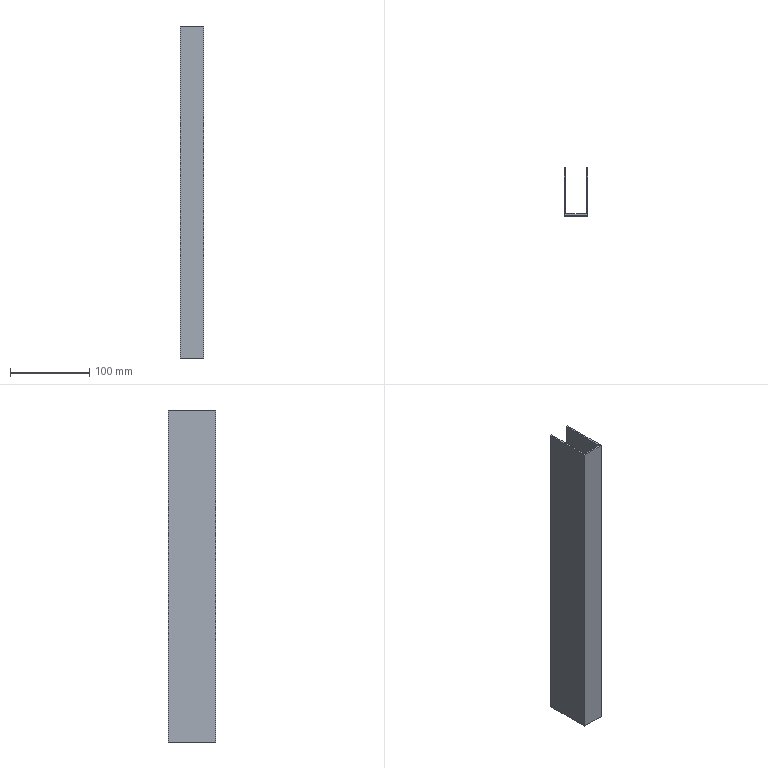Part | SolidWorks | features Extrusion 1, Shell 1 | 1 solid | 10 faces | box 30 x 60 x 418 mm | volume 122056 mm3 | plane 10
STEP:
#1=CARTESIAN_POINT('',(13.,30.,209.));
#2=VERTEX_POINT('',#1);
#3=CARTESIAN_POINT('',(13.,30.,-209.));
#4=VERTEX_POINT('',#3);
#5=CARTESIAN_POINT('',(13.,30.,209.));
#6=DIRECTION('',(0.,0.,-1.));
#7=VECTOR('',#6,1000.);
#8=LINE('',#5,#7);
#9=EDGE_CURVE('',#2,#4,#8,.T.);
#10=ORIENTED_EDGE('',*,*,#9,.F.);
#11=CARTESIAN_POINT('',(15.,30.,209.));
#12=VERTEX_POINT('',#11);
#13=CARTESIAN_POINT('',(-15.,30.,209.));
#14=DIRECTION('',(-1.,0.,0.));
#15=VECTOR('',#14,1000.);
#16=LINE('',#13,#15);
#17=EDGE_CURVE('',#12,#2,#16,.T.);
#18=ORIENTED_EDGE('',*,*,#17,.F.);
#19=CARTESIAN_POINT('',(15.,30.,-209.));
#20=VERTEX_POINT('',#19);
#21=CARTESIAN_POINT('',(15.,30.,209.));
#22=DIRECTION('',(0.,0.,-1.));
#23=VECTOR('',#22,1000.);
#24=LINE('',#21,#23);
#25=EDGE_CURVE('',#12,#20,#24,.T.);
#26=ORIENTED_EDGE('',*,*,#25,.T.);
#27=CARTESIAN_POINT('',(-15.,30.,-209.));
#28=DIRECTION('',(-1.,0.,0.));
#29=VECTOR('',#28,1000.);
#30=LINE('',#27,#29);
#31=EDGE_CURVE('',#20,#4,#30,.T.);
#32=ORIENTED_EDGE('',*,*,#31,.T.);
#33=EDGE_LOOP('',(#10,#18,#26,#32));
#34=FACE_OUTER_BOUND('',#33,.T.);
#35=CARTESIAN_POINT('',(-15.,30.,209.));
#36=DIRECTION('',(0.,-1.,0.));
#37=DIRECTION('',(0.,0.,-1.));
#38=AXIS2_PLACEMENT_3D('',#35,#36,#37);
#39=PLANE('',#38);
#40=ADVANCED_FACE('',(#34),#39,.F.);
#41=CARTESIAN_POINT('',(13.,-28.,209.));
#42=VERTEX_POINT('',#41);
#43=CARTESIAN_POINT('',(13.,0.,209.));
#44=DIRECTION('',(0.,1.,0.));
#45=VECTOR('',#44,1000.);
#46=LINE('',#43,#45);
#47=EDGE_CURVE('',#42,#2,#46,.T.);
#48=ORIENTED_EDGE('',*,*,#47,.F.);
#49=CARTESIAN_POINT('',(-13.,-28.,209.));
#50=VERTEX_POINT('',#49);
#51=CARTESIAN_POINT('',(0.,-28.,209.));
#52=DIRECTION('',(1.,0.,0.));
#53=VECTOR('',#52,1000.);
#54=LINE('',#51,#53);
#55=EDGE_CURVE('',#50,#42,#54,.T.);
#56=ORIENTED_EDGE('',*,*,#55,.F.);
#57=CARTESIAN_POINT('',(-13.,30.,209.));
#58=VERTEX_POINT('',#57);
#59=CARTESIAN_POINT('',(-13.,0.,209.));
#60=DIRECTION('',(0.,-1.,0.));
#61=VECTOR('',#60,1000.);
#62=LINE('',#59,#61);
#63=EDGE_CURVE('',#58,#50,#62,.T.);
#64=ORIENTED_EDGE('',*,*,#63,.F.);
#65=CARTESIAN_POINT('',(-15.,30.,209.));
#66=VERTEX_POINT('',#65);
#67=CARTESIAN_POINT('',(-15.,30.,209.));
#68=DIRECTION('',(-1.,0.,0.));
#69=VECTOR('',#68,1000.);
#70=LINE('',#67,#69);
#71=EDGE_CURVE('',#58,#66,#70,.T.);
#72=ORIENTED_EDGE('',*,*,#71,.T.);
#73=CARTESIAN_POINT('',(-15.,-30.,209.));
#74=VERTEX_POINT('',#73);
#75=CARTESIAN_POINT('',(-15.,-30.,209.));
#76=DIRECTION('',(0.,-1.,0.));
#77=VECTOR('',#76,1000.);
#78=LINE('',#75,#77);
#79=EDGE_CURVE('',#66,#74,#78,.T.);
#80=ORIENTED_EDGE('',*,*,#79,.T.);
#81=CARTESIAN_POINT('',(15.,-30.,209.));
#82=VERTEX_POINT('',#81);
#83=CARTESIAN_POINT('',(-15.,-30.,209.));
#84=DIRECTION('',(1.,0.,0.));
#85=VECTOR('',#84,1000.);
#86=LINE('',#83,#85);
#87=EDGE_CURVE('',#74,#82,#86,.T.);
#88=ORIENTED_EDGE('',*,*,#87,.T.);
#89=CARTESIAN_POINT('',(15.,-30.,209.));
#90=DIRECTION('',(0.,1.,0.));
#91=VECTOR('',#90,1000.);
#92=LINE('',#89,#91);
#93=EDGE_CURVE('',#82,#12,#92,.T.);
#94=ORIENTED_EDGE('',*,*,#93,.T.);
#95=ORIENTED_EDGE('',*,*,#17,.T.);
#96=EDGE_LOOP('',(#48,#56,#64,#72,#80,#88,#94,#95));
#97=FACE_OUTER_BOUND('',#96,.T.);
#98=CARTESIAN_POINT('',(0.,0.,209.));
#99=DIRECTION('',(0.,0.,-1.));
#100=DIRECTION('',(-1.,0.,0.));
#101=AXIS2_PLACEMENT_3D('',#98,#99,#100);
#102=PLANE('',#101);
#103=ADVANCED_FACE('',(#97),#102,.F.);
#104=CARTESIAN_POINT('',(-13.,-28.,-209.));
#105=VERTEX_POINT('',#104);
#106=CARTESIAN_POINT('',(13.,-28.,-209.));
#107=VERTEX_POINT('',#106);
#108=CARTESIAN_POINT('',(0.,-28.,-209.));
#109=DIRECTION('',(1.,0.,0.));
#110=VECTOR('',#109,1000.);
#111=LINE('',#108,#110);
#112=EDGE_CURVE('',#105,#107,#111,.T.);
#113=ORIENTED_EDGE('',*,*,#112,.T.);
#114=CARTESIAN_POINT('',(13.,0.,-209.));
#115=DIRECTION('',(0.,1.,0.));
#116=VECTOR('',#115,1000.);
#117=LINE('',#114,#116);
#118=EDGE_CURVE('',#107,#4,#117,.T.);
#119=ORIENTED_EDGE('',*,*,#118,.T.);
#120=ORIENTED_EDGE('',*,*,#31,.F.);
#121=CARTESIAN_POINT('',(15.,-30.,-209.));
#122=VERTEX_POINT('',#121);
#123=CARTESIAN_POINT('',(15.,-30.,-209.));
#124=DIRECTION('',(0.,1.,0.));
#125=VECTOR('',#124,1000.);
#126=LINE('',#123,#125);
#127=EDGE_CURVE('',#122,#20,#126,.T.);
#128=ORIENTED_EDGE('',*,*,#127,.F.);
#129=CARTESIAN_POINT('',(-15.,-30.,-209.));
#130=VERTEX_POINT('',#129);
#131=CARTESIAN_POINT('',(-15.,-30.,-209.));
#132=DIRECTION('',(1.,0.,0.));
#133=VECTOR('',#132,1000.);
#134=LINE('',#131,#133);
#135=EDGE_CURVE('',#130,#122,#134,.T.);
#136=ORIENTED_EDGE('',*,*,#135,.F.);
#137=CARTESIAN_POINT('',(-15.,30.,-209.));
#138=VERTEX_POINT('',#137);
#139=CARTESIAN_POINT('',(-15.,-30.,-209.));
#140=DIRECTION('',(0.,-1.,0.));
#141=VECTOR('',#140,1000.);
#142=LINE('',#139,#141);
#143=EDGE_CURVE('',#138,#130,#142,.T.);
#144=ORIENTED_EDGE('',*,*,#143,.F.);
#145=CARTESIAN_POINT('',(-13.,30.,-209.));
#146=VERTEX_POINT('',#145);
#147=CARTESIAN_POINT('',(-15.,30.,-209.));
#148=DIRECTION('',(-1.,0.,0.));
#149=VECTOR('',#148,1000.);
#150=LINE('',#147,#149);
#151=EDGE_CURVE('',#146,#138,#150,.T.);
#152=ORIENTED_EDGE('',*,*,#151,.F.);
#153=CARTESIAN_POINT('',(-13.,0.,-209.));
#154=DIRECTION('',(0.,-1.,0.));
#155=VECTOR('',#154,1000.);
#156=LINE('',#153,#155);
#157=EDGE_CURVE('',#146,#105,#156,.T.);
#158=ORIENTED_EDGE('',*,*,#157,.T.);
#159=EDGE_LOOP('',(#113,#119,#120,#128,#136,#144,#152,#158));
#160=FACE_OUTER_BOUND('',#159,.T.);
#161=CARTESIAN_POINT('',(0.,0.,-209.));
#162=DIRECTION('',(0.,0.,-1.));
#163=DIRECTION('',(-1.,0.,0.));
#164=AXIS2_PLACEMENT_3D('',#161,#162,#163);
#165=PLANE('',#164);
#166=ADVANCED_FACE('',(#160),#165,.T.);
#167=ORIENTED_EDGE('',*,*,#127,.T.);
#168=ORIENTED_EDGE('',*,*,#25,.F.);
#169=ORIENTED_EDGE('',*,*,#93,.F.);
#170=CARTESIAN_POINT('',(15.,-30.,209.));
#171=DIRECTION('',(0.,0.,-1.));
#172=VECTOR('',#171,1000.);
#173=LINE('',#170,#172);
#174=EDGE_CURVE('',#82,#122,#173,.T.);
#175=ORIENTED_EDGE('',*,*,#174,.T.);
#176=EDGE_LOOP('',(#167,#168,#169,#175));
#177=FACE_OUTER_BOUND('',#176,.T.);
#178=CARTESIAN_POINT('',(15.,-30.,209.));
#179=DIRECTION('',(-1.,0.,0.));
#180=DIRECTION('',(0.,0.,1.));
#181=AXIS2_PLACEMENT_3D('',#178,#179,#180);
#182=PLANE('',#181);
#183=ADVANCED_FACE('',(#177),#182,.F.);
#184=ORIENTED_EDGE('',*,*,#71,.F.);
#185=CARTESIAN_POINT('',(-13.,30.,209.));
#186=DIRECTION('',(0.,0.,-1.));
#187=VECTOR('',#186,1000.);
#188=LINE('',#185,#187);
#189=EDGE_CURVE('',#58,#146,#188,.T.);
#190=ORIENTED_EDGE('',*,*,#189,.T.);
#191=ORIENTED_EDGE('',*,*,#151,.T.);
#192=CARTESIAN_POINT('',(-15.,30.,209.));
#193=DIRECTION('',(0.,0.,-1.));
#194=VECTOR('',#193,1000.);
#195=LINE('',#192,#194);
#196=EDGE_CURVE('',#66,#138,#195,.T.);
#197=ORIENTED_EDGE('',*,*,#196,.F.);
#198=EDGE_LOOP('',(#184,#190,#191,#197));
#199=FACE_OUTER_BOUND('',#198,.T.);
#200=CARTESIAN_POINT('',(-15.,30.,209.));
#201=DIRECTION('',(0.,-1.,0.));
#202=DIRECTION('',(0.,0.,-1.));
#203=AXIS2_PLACEMENT_3D('',#200,#201,#202);
#204=PLANE('',#203);
#205=ADVANCED_FACE('',(#199),#204,.F.);
#206=ORIENTED_EDGE('',*,*,#143,.T.);
#207=CARTESIAN_POINT('',(-15.,-30.,209.));
#208=DIRECTION('',(0.,0.,-1.));
#209=VECTOR('',#208,1000.);
#210=LINE('',#207,#209);
#211=EDGE_CURVE('',#74,#130,#210,.T.);
#212=ORIENTED_EDGE('',*,*,#211,.F.);
#213=ORIENTED_EDGE('',*,*,#79,.F.);
#214=ORIENTED_EDGE('',*,*,#196,.T.);
#215=EDGE_LOOP('',(#206,#212,#213,#214));
#216=FACE_OUTER_BOUND('',#215,.T.);
#217=CARTESIAN_POINT('',(-15.,-30.,209.));
#218=DIRECTION('',(1.,0.,0.));
#219=DIRECTION('',(0.,0.,-1.));
#220=AXIS2_PLACEMENT_3D('',#217,#218,#219);
#221=PLANE('',#220);
#222=ADVANCED_FACE('',(#216),#221,.F.);
#223=ORIENTED_EDGE('',*,*,#135,.T.);
#224=ORIENTED_EDGE('',*,*,#174,.F.);
#225=ORIENTED_EDGE('',*,*,#87,.F.);
#226=ORIENTED_EDGE('',*,*,#211,.T.);
#227=EDGE_LOOP('',(#223,#224,#225,#226));
#228=FACE_OUTER_BOUND('',#227,.T.);
#229=CARTESIAN_POINT('',(-15.,-30.,209.));
#230=DIRECTION('',(0.,1.,0.));
#231=DIRECTION('',(0.,0.,1.));
#232=AXIS2_PLACEMENT_3D('',#229,#230,#231);
#233=PLANE('',#232);
#234=ADVANCED_FACE('',(#228),#233,.F.);
#235=ORIENTED_EDGE('',*,*,#118,.F.);
#236=CARTESIAN_POINT('',(13.,-28.,209.));
#237=DIRECTION('',(0.,0.,-1.));
#238=VECTOR('',#237,1000.);
#239=LINE('',#236,#238);
#240=EDGE_CURVE('',#42,#107,#239,.T.);
#241=ORIENTED_EDGE('',*,*,#240,.F.);
#242=ORIENTED_EDGE('',*,*,#47,.T.);
#243=ORIENTED_EDGE('',*,*,#9,.T.);
#244=EDGE_LOOP('',(#235,#241,#242,#243));
#245=FACE_OUTER_BOUND('',#244,.T.);
#246=CARTESIAN_POINT('',(13.,-30.,209.));
#247=DIRECTION('',(-1.,0.,0.));
#248=DIRECTION('',(0.,0.,1.));
#249=AXIS2_PLACEMENT_3D('',#246,#247,#248);
#250=PLANE('',#249);
#251=ADVANCED_FACE('',(#245),#250,.T.);
#252=ORIENTED_EDGE('',*,*,#157,.F.);
#253=ORIENTED_EDGE('',*,*,#189,.F.);
#254=ORIENTED_EDGE('',*,*,#63,.T.);
#255=CARTESIAN_POINT('',(-13.,-28.,209.));
#256=DIRECTION('',(0.,0.,-1.));
#257=VECTOR('',#256,1000.);
#258=LINE('',#255,#257);
#259=EDGE_CURVE('',#50,#105,#258,.T.);
#260=ORIENTED_EDGE('',*,*,#259,.T.);
#261=EDGE_LOOP('',(#252,#253,#254,#260));
#262=FACE_OUTER_BOUND('',#261,.T.);
#263=CARTESIAN_POINT('',(-13.,-30.,209.));
#264=DIRECTION('',(1.,0.,0.));
#265=DIRECTION('',(0.,0.,-1.));
#266=AXIS2_PLACEMENT_3D('',#263,#264,#265);
#267=PLANE('',#266);
#268=ADVANCED_FACE('',(#262),#267,.T.);
#269=ORIENTED_EDGE('',*,*,#112,.F.);
#270=ORIENTED_EDGE('',*,*,#259,.F.);
#271=ORIENTED_EDGE('',*,*,#55,.T.);
#272=ORIENTED_EDGE('',*,*,#240,.T.);
#273=EDGE_LOOP('',(#269,#270,#271,#272));
#274=FACE_OUTER_BOUND('',#273,.T.);
#275=CARTESIAN_POINT('',(-15.,-28.,209.));
#276=DIRECTION('',(0.,1.,0.));
#277=DIRECTION('',(0.,0.,1.));
#278=AXIS2_PLACEMENT_3D('',#275,#276,#277);
#279=PLANE('',#278);
#280=ADVANCED_FACE('',(#274),#279,.T.);
#281=CLOSED_SHELL('',(#40,#103,#166,#183,#205,#222,#234,#251,#268,#280));
#282=MANIFOLD_SOLID_BREP('',#281);
#283=CARTESIAN_POINT('',(0.,0.,0.));
#284=DIRECTION('',(0.,0.,1.));
#285=DIRECTION('',(1.,0.,0.));
#286=AXIS2_PLACEMENT_3D('',#283,#284,#285);
#287=(LENGTH_UNIT()NAMED_UNIT(*)SI_UNIT(.MILLI.,.METRE.));
#288=UNCERTAINTY_MEASURE_WITH_UNIT(LENGTH_MEASURE(0.00001),#287,'','');
#289=(NAMED_UNIT(*)PLANE_ANGLE_UNIT()SI_UNIT($,.RADIAN.));
#290=(NAMED_UNIT(*)SI_UNIT($,.STERADIAN.)SOLID_ANGLE_UNIT());
#291=(GEOMETRIC_REPRESENTATION_CONTEXT(3)GLOBAL_UNCERTAINTY_ASSIGNED_CONTEXT((#288))GLOBAL_UNIT_ASSIGNED_CONTEXT((#287,#289,#290))REPRESENTATION_CONTEXT('',''));
#292=ADVANCED_BREP_SHAPE_REPRESENTATION('',(#282,#286),#291);